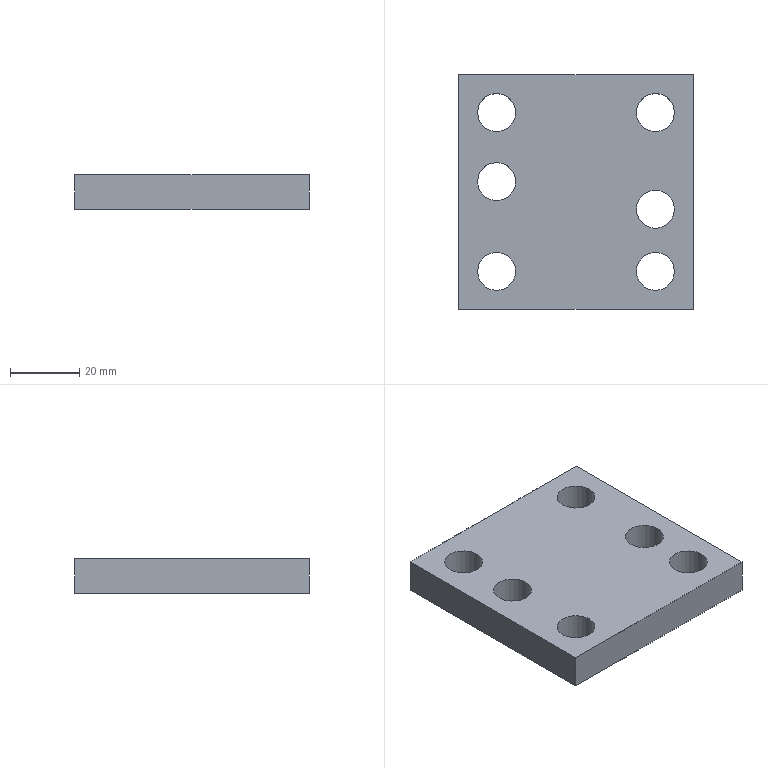Part | NX | features solid 2 | 1 solid | 12 faces | box 68 x 68 x 10 mm | volume 40538 mm3 | plane 6 | cylinder 6 | commonest cylinder face diameters 11 x6
STEP:
#1=CARTESIAN_POINT('',(1122.079,-107.904,88.));
#2=VERTEX_POINT('',#1);
#3=CARTESIAN_POINT('',(1122.079,-107.904,78.));
#4=VERTEX_POINT('',#3);
#5=CARTESIAN_POINT('',(1122.079,-107.904,78.));
#6=DIRECTION('',(0.,0.,1.));
#7=VECTOR('',#6,1000.);
#8=LINE('',#5,#7);
#9=EDGE_CURVE('',#2,#4,#8,.F.);
#10=ORIENTED_EDGE('',*,*,#9,.T.);
#11=CARTESIAN_POINT('',(1054.079,-107.904,78.));
#12=VERTEX_POINT('',#11);
#13=CARTESIAN_POINT('',(1088.079,-107.904,78.));
#14=DIRECTION('',(-1.,0.,0.));
#15=VECTOR('',#14,1000.);
#16=LINE('',#13,#15);
#17=EDGE_CURVE('',#12,#4,#16,.F.);
#18=ORIENTED_EDGE('',*,*,#17,.F.);
#19=CARTESIAN_POINT('',(1054.079,-107.904,88.));
#20=VERTEX_POINT('',#19);
#21=CARTESIAN_POINT('',(1054.079,-107.904,78.));
#22=DIRECTION('',(0.,0.,1.));
#23=VECTOR('',#22,1000.);
#24=LINE('',#21,#23);
#25=EDGE_CURVE('',#20,#12,#24,.F.);
#26=ORIENTED_EDGE('',*,*,#25,.F.);
#27=CARTESIAN_POINT('',(287.,-107.904,88.));
#28=DIRECTION('',(-1.,0.,0.));
#29=VECTOR('',#28,1000.);
#30=LINE('',#27,#29);
#31=EDGE_CURVE('',#20,#2,#30,.F.);
#32=ORIENTED_EDGE('',*,*,#31,.T.);
#33=EDGE_LOOP('',(#10,#18,#26,#32));
#34=FACE_BOUND('',#33,.T.);
#35=CARTESIAN_POINT('',(1088.079,-107.904,78.));
#36=DIRECTION('',(0.,-1.,0.));
#37=DIRECTION('',(-1.,0.,0.));
#38=AXIS2_PLACEMENT_3D('',#35,#36,#37);
#39=PLANE('',#38);
#40=ADVANCED_FACE('',(#34),#39,.F.);
#41=ORIENTED_EDGE('',*,*,#25,.T.);
#42=CARTESIAN_POINT('',(1054.079,-175.904,78.));
#43=VERTEX_POINT('',#42);
#44=CARTESIAN_POINT('',(1054.079,-141.904,78.));
#45=DIRECTION('',(0.,-1.,0.));
#46=VECTOR('',#45,1000.);
#47=LINE('',#44,#46);
#48=EDGE_CURVE('',#43,#12,#47,.F.);
#49=ORIENTED_EDGE('',*,*,#48,.F.);
#50=CARTESIAN_POINT('',(1054.079,-175.904,88.));
#51=VERTEX_POINT('',#50);
#52=CARTESIAN_POINT('',(1054.079,-175.904,78.));
#53=DIRECTION('',(0.,0.,1.));
#54=VECTOR('',#53,1000.);
#55=LINE('',#52,#54);
#56=EDGE_CURVE('',#51,#43,#55,.F.);
#57=ORIENTED_EDGE('',*,*,#56,.F.);
#58=CARTESIAN_POINT('',(1054.079,-0.000000688,88.));
#59=DIRECTION('',(0.,1.,0.));
#60=VECTOR('',#59,1000.);
#61=LINE('',#58,#60);
#62=EDGE_CURVE('',#51,#20,#61,.T.);
#63=ORIENTED_EDGE('',*,*,#62,.T.);
#64=EDGE_LOOP('',(#41,#49,#57,#63));
#65=FACE_BOUND('',#64,.T.);
#66=CARTESIAN_POINT('',(1054.079,-141.904,78.));
#67=DIRECTION('',(1.,0.,0.));
#68=DIRECTION('',(0.,-1.,0.));
#69=AXIS2_PLACEMENT_3D('',#66,#67,#68);
#70=PLANE('',#69);
#71=ADVANCED_FACE('',(#65),#70,.F.);
#72=ORIENTED_EDGE('',*,*,#56,.T.);
#73=CARTESIAN_POINT('',(1122.079,-175.904,78.));
#74=VERTEX_POINT('',#73);
#75=CARTESIAN_POINT('',(1088.079,-175.904,78.));
#76=DIRECTION('',(1.,0.,0.));
#77=VECTOR('',#76,1000.);
#78=LINE('',#75,#77);
#79=EDGE_CURVE('',#74,#43,#78,.F.);
#80=ORIENTED_EDGE('',*,*,#79,.F.);
#81=CARTESIAN_POINT('',(1122.079,-175.904,88.));
#82=VERTEX_POINT('',#81);
#83=CARTESIAN_POINT('',(1122.079,-175.904,78.));
#84=DIRECTION('',(0.,0.,1.));
#85=VECTOR('',#84,1000.);
#86=LINE('',#83,#85);
#87=EDGE_CURVE('',#82,#74,#86,.F.);
#88=ORIENTED_EDGE('',*,*,#87,.F.);
#89=CARTESIAN_POINT('',(287.,-175.904,88.));
#90=DIRECTION('',(-1.,0.,0.));
#91=VECTOR('',#90,1000.);
#92=LINE('',#89,#91);
#93=EDGE_CURVE('',#82,#51,#92,.T.);
#94=ORIENTED_EDGE('',*,*,#93,.T.);
#95=EDGE_LOOP('',(#72,#80,#88,#94));
#96=FACE_BOUND('',#95,.T.);
#97=CARTESIAN_POINT('',(1088.079,-175.904,78.));
#98=DIRECTION('',(0.,1.,0.));
#99=DIRECTION('',(1.,0.,0.));
#100=AXIS2_PLACEMENT_3D('',#97,#98,#99);
#101=PLANE('',#100);
#102=ADVANCED_FACE('',(#96),#101,.F.);
#103=CARTESIAN_POINT('',(1105.579,-146.904,78.));
#104=VERTEX_POINT('',#103);
#105=CARTESIAN_POINT('',(1111.079,-146.904,78.));
#106=DIRECTION('',(0.,0.,-1.));
#107=DIRECTION('',(-1.,0.,0.));
#108=AXIS2_PLACEMENT_3D('',#105,#106,#107);
#109=CIRCLE('',#108,5.5);
#110=EDGE_CURVE('',#104,#104,#109,.T.);
#111=ORIENTED_EDGE('',*,*,#110,.T.);
#112=EDGE_LOOP('',(#111));
#113=FACE_BOUND('',#112,.T.);
#114=CARTESIAN_POINT('',(1105.579,-146.904,88.));
#115=VERTEX_POINT('',#114);
#116=CARTESIAN_POINT('',(1111.079,-146.904,88.));
#117=DIRECTION('',(0.,0.,-1.));
#118=DIRECTION('',(-1.,0.,0.));
#119=AXIS2_PLACEMENT_3D('',#116,#117,#118);
#120=CIRCLE('',#119,5.5);
#121=EDGE_CURVE('',#115,#115,#120,.T.);
#122=ORIENTED_EDGE('',*,*,#121,.F.);
#123=EDGE_LOOP('',(#122));
#124=FACE_BOUND('',#123,.T.);
#125=CARTESIAN_POINT('',(1111.079,-146.904,78.));
#126=DIRECTION('',(0.,0.,-1.));
#127=DIRECTION('',(-1.,0.,0.));
#128=AXIS2_PLACEMENT_3D('',#125,#126,#127);
#129=CYLINDRICAL_SURFACE('',#128,5.5);
#130=ADVANCED_FACE('',(#113,#124),#129,.F.);
#131=CARTESIAN_POINT('',(1059.579,-138.904,78.));
#132=VERTEX_POINT('',#131);
#133=CARTESIAN_POINT('',(1065.079,-138.904,78.));
#134=DIRECTION('',(0.,0.,-1.));
#135=DIRECTION('',(-1.,0.,0.));
#136=AXIS2_PLACEMENT_3D('',#133,#134,#135);
#137=CIRCLE('',#136,5.5);
#138=EDGE_CURVE('',#132,#132,#137,.F.);
#139=ORIENTED_EDGE('',*,*,#138,.F.);
#140=EDGE_LOOP('',(#139));
#141=FACE_BOUND('',#140,.T.);
#142=CARTESIAN_POINT('',(1059.579,-138.904,88.));
#143=VERTEX_POINT('',#142);
#144=CARTESIAN_POINT('',(1065.079,-138.904,88.));
#145=DIRECTION('',(0.,0.,-1.));
#146=DIRECTION('',(-1.,0.,0.));
#147=AXIS2_PLACEMENT_3D('',#144,#145,#146);
#148=CIRCLE('',#147,5.5);
#149=EDGE_CURVE('',#143,#143,#148,.F.);
#150=ORIENTED_EDGE('',*,*,#149,.T.);
#151=EDGE_LOOP('',(#150));
#152=FACE_BOUND('',#151,.T.);
#153=CARTESIAN_POINT('',(1065.079,-138.904,78.));
#154=DIRECTION('',(0.,0.,-1.));
#155=DIRECTION('',(-1.,0.,0.));
#156=AXIS2_PLACEMENT_3D('',#153,#154,#155);
#157=CYLINDRICAL_SURFACE('',#156,5.5);
#158=ADVANCED_FACE('',(#141,#152),#157,.F.);
#159=CARTESIAN_POINT('',(1105.579,-118.904,78.));
#160=VERTEX_POINT('',#159);
#161=CARTESIAN_POINT('',(1111.079,-118.904,78.));
#162=DIRECTION('',(0.,0.,-1.));
#163=DIRECTION('',(-1.,0.,0.));
#164=AXIS2_PLACEMENT_3D('',#161,#162,#163);
#165=CIRCLE('',#164,5.5);
#166=EDGE_CURVE('',#160,#160,#165,.T.);
#167=ORIENTED_EDGE('',*,*,#166,.T.);
#168=EDGE_LOOP('',(#167));
#169=FACE_BOUND('',#168,.T.);
#170=CARTESIAN_POINT('',(1105.579,-118.904,88.));
#171=VERTEX_POINT('',#170);
#172=CARTESIAN_POINT('',(1111.079,-118.904,88.));
#173=DIRECTION('',(0.,0.,-1.));
#174=DIRECTION('',(-1.,0.,0.));
#175=AXIS2_PLACEMENT_3D('',#172,#173,#174);
#176=CIRCLE('',#175,5.5);
#177=EDGE_CURVE('',#171,#171,#176,.T.);
#178=ORIENTED_EDGE('',*,*,#177,.F.);
#179=EDGE_LOOP('',(#178));
#180=FACE_BOUND('',#179,.T.);
#181=CARTESIAN_POINT('',(1111.079,-118.904,78.));
#182=DIRECTION('',(0.,0.,-1.));
#183=DIRECTION('',(-1.,0.,0.));
#184=AXIS2_PLACEMENT_3D('',#181,#182,#183);
#185=CYLINDRICAL_SURFACE('',#184,5.5);
#186=ADVANCED_FACE('',(#169,#180),#185,.F.);
#187=CARTESIAN_POINT('',(1105.579,-164.904,78.));
#188=VERTEX_POINT('',#187);
#189=CARTESIAN_POINT('',(1111.079,-164.904,78.));
#190=DIRECTION('',(0.,0.,-1.));
#191=DIRECTION('',(-1.,0.,0.));
#192=AXIS2_PLACEMENT_3D('',#189,#190,#191);
#193=CIRCLE('',#192,5.5);
#194=EDGE_CURVE('',#188,#188,#193,.T.);
#195=ORIENTED_EDGE('',*,*,#194,.T.);
#196=EDGE_LOOP('',(#195));
#197=FACE_BOUND('',#196,.T.);
#198=CARTESIAN_POINT('',(1105.579,-164.904,88.));
#199=VERTEX_POINT('',#198);
#200=CARTESIAN_POINT('',(1111.079,-164.904,88.));
#201=DIRECTION('',(0.,0.,-1.));
#202=DIRECTION('',(-1.,0.,0.));
#203=AXIS2_PLACEMENT_3D('',#200,#201,#202);
#204=CIRCLE('',#203,5.5);
#205=EDGE_CURVE('',#199,#199,#204,.T.);
#206=ORIENTED_EDGE('',*,*,#205,.F.);
#207=EDGE_LOOP('',(#206));
#208=FACE_BOUND('',#207,.T.);
#209=CARTESIAN_POINT('',(1111.079,-164.904,78.));
#210=DIRECTION('',(0.,0.,-1.));
#211=DIRECTION('',(-1.,0.,0.));
#212=AXIS2_PLACEMENT_3D('',#209,#210,#211);
#213=CYLINDRICAL_SURFACE('',#212,5.5);
#214=ADVANCED_FACE('',(#197,#208),#213,.F.);
#215=CARTESIAN_POINT('',(1059.579,-164.904,78.));
#216=VERTEX_POINT('',#215);
#217=CARTESIAN_POINT('',(1065.079,-164.904,78.));
#218=DIRECTION('',(0.,0.,-1.));
#219=DIRECTION('',(-1.,0.,0.));
#220=AXIS2_PLACEMENT_3D('',#217,#218,#219);
#221=CIRCLE('',#220,5.5);
#222=EDGE_CURVE('',#216,#216,#221,.T.);
#223=ORIENTED_EDGE('',*,*,#222,.T.);
#224=EDGE_LOOP('',(#223));
#225=FACE_BOUND('',#224,.T.);
#226=CARTESIAN_POINT('',(1059.579,-164.904,88.));
#227=VERTEX_POINT('',#226);
#228=CARTESIAN_POINT('',(1065.079,-164.904,88.));
#229=DIRECTION('',(0.,0.,-1.));
#230=DIRECTION('',(-1.,0.,0.));
#231=AXIS2_PLACEMENT_3D('',#228,#229,#230);
#232=CIRCLE('',#231,5.5);
#233=EDGE_CURVE('',#227,#227,#232,.T.);
#234=ORIENTED_EDGE('',*,*,#233,.F.);
#235=EDGE_LOOP('',(#234));
#236=FACE_BOUND('',#235,.T.);
#237=CARTESIAN_POINT('',(1065.079,-164.904,78.));
#238=DIRECTION('',(0.,0.,-1.));
#239=DIRECTION('',(-1.,0.,0.));
#240=AXIS2_PLACEMENT_3D('',#237,#238,#239);
#241=CYLINDRICAL_SURFACE('',#240,5.5);
#242=ADVANCED_FACE('',(#225,#236),#241,.F.);
#243=CARTESIAN_POINT('',(1059.579,-118.904,78.));
#244=VERTEX_POINT('',#243);
#245=CARTESIAN_POINT('',(1065.079,-118.904,78.));
#246=DIRECTION('',(0.,0.,-1.));
#247=DIRECTION('',(-1.,0.,0.));
#248=AXIS2_PLACEMENT_3D('',#245,#246,#247);
#249=CIRCLE('',#248,5.5);
#250=EDGE_CURVE('',#244,#244,#249,.F.);
#251=ORIENTED_EDGE('',*,*,#250,.F.);
#252=EDGE_LOOP('',(#251));
#253=FACE_BOUND('',#252,.T.);
#254=CARTESIAN_POINT('',(1059.579,-118.904,88.));
#255=VERTEX_POINT('',#254);
#256=CARTESIAN_POINT('',(1065.079,-118.904,88.));
#257=DIRECTION('',(0.,0.,-1.));
#258=DIRECTION('',(-1.,0.,0.));
#259=AXIS2_PLACEMENT_3D('',#256,#257,#258);
#260=CIRCLE('',#259,5.5);
#261=EDGE_CURVE('',#255,#255,#260,.F.);
#262=ORIENTED_EDGE('',*,*,#261,.T.);
#263=EDGE_LOOP('',(#262));
#264=FACE_BOUND('',#263,.T.);
#265=CARTESIAN_POINT('',(1065.079,-118.904,78.));
#266=DIRECTION('',(0.,0.,-1.));
#267=DIRECTION('',(-1.,0.,0.));
#268=AXIS2_PLACEMENT_3D('',#265,#266,#267);
#269=CYLINDRICAL_SURFACE('',#268,5.5);
#270=ADVANCED_FACE('',(#253,#264),#269,.F.);
#271=CARTESIAN_POINT('',(1122.079,-0.000000688,88.));
#272=DIRECTION('',(0.,1.,0.));
#273=VECTOR('',#272,1000.);
#274=LINE('',#271,#273);
#275=EDGE_CURVE('',#2,#82,#274,.F.);
#276=ORIENTED_EDGE('',*,*,#275,.T.);
#277=ORIENTED_EDGE('',*,*,#87,.T.);
#278=CARTESIAN_POINT('',(1122.079,-141.904,78.));
#279=DIRECTION('',(0.,1.,0.));
#280=VECTOR('',#279,1000.);
#281=LINE('',#278,#280);
#282=EDGE_CURVE('',#4,#74,#281,.F.);
#283=ORIENTED_EDGE('',*,*,#282,.F.);
#284=ORIENTED_EDGE('',*,*,#9,.F.);
#285=EDGE_LOOP('',(#276,#277,#283,#284));
#286=FACE_BOUND('',#285,.T.);
#287=CARTESIAN_POINT('',(1122.079,-141.904,78.));
#288=DIRECTION('',(-1.,0.,0.));
#289=DIRECTION('',(0.,1.,0.));
#290=AXIS2_PLACEMENT_3D('',#287,#288,#289);
#291=PLANE('',#290);
#292=ADVANCED_FACE('',(#286),#291,.F.);
#293=ORIENTED_EDGE('',*,*,#110,.F.);
#294=EDGE_LOOP('',(#293));
#295=FACE_BOUND('',#294,.T.);
#296=ORIENTED_EDGE('',*,*,#138,.T.);
#297=EDGE_LOOP('',(#296));
#298=FACE_BOUND('',#297,.T.);
#299=ORIENTED_EDGE('',*,*,#166,.F.);
#300=EDGE_LOOP('',(#299));
#301=FACE_BOUND('',#300,.T.);
#302=ORIENTED_EDGE('',*,*,#194,.F.);
#303=EDGE_LOOP('',(#302));
#304=FACE_BOUND('',#303,.T.);
#305=ORIENTED_EDGE('',*,*,#222,.F.);
#306=EDGE_LOOP('',(#305));
#307=FACE_BOUND('',#306,.T.);
#308=ORIENTED_EDGE('',*,*,#250,.T.);
#309=EDGE_LOOP('',(#308));
#310=FACE_BOUND('',#309,.T.);
#311=ORIENTED_EDGE('',*,*,#79,.T.);
#312=ORIENTED_EDGE('',*,*,#48,.T.);
#313=ORIENTED_EDGE('',*,*,#17,.T.);
#314=ORIENTED_EDGE('',*,*,#282,.T.);
#315=EDGE_LOOP('',(#311,#312,#313,#314));
#316=FACE_BOUND('',#315,.T.);
#317=CARTESIAN_POINT('',(287.,-0.000000688,78.));
#318=DIRECTION('',(0.,0.,-1.));
#319=DIRECTION('',(-1.,0.,0.));
#320=AXIS2_PLACEMENT_3D('',#317,#318,#319);
#321=PLANE('',#320);
#322=ADVANCED_FACE('',(#295,#298,#301,#304,#307,#310,#316),#321,.T.);
#323=ORIENTED_EDGE('',*,*,#121,.T.);
#324=EDGE_LOOP('',(#323));
#325=FACE_BOUND('',#324,.T.);
#326=ORIENTED_EDGE('',*,*,#149,.F.);
#327=EDGE_LOOP('',(#326));
#328=FACE_BOUND('',#327,.T.);
#329=ORIENTED_EDGE('',*,*,#177,.T.);
#330=EDGE_LOOP('',(#329));
#331=FACE_BOUND('',#330,.T.);
#332=ORIENTED_EDGE('',*,*,#205,.T.);
#333=EDGE_LOOP('',(#332));
#334=FACE_BOUND('',#333,.T.);
#335=ORIENTED_EDGE('',*,*,#233,.T.);
#336=EDGE_LOOP('',(#335));
#337=FACE_BOUND('',#336,.T.);
#338=ORIENTED_EDGE('',*,*,#261,.F.);
#339=EDGE_LOOP('',(#338));
#340=FACE_BOUND('',#339,.T.);
#341=ORIENTED_EDGE('',*,*,#93,.F.);
#342=ORIENTED_EDGE('',*,*,#275,.F.);
#343=ORIENTED_EDGE('',*,*,#31,.F.);
#344=ORIENTED_EDGE('',*,*,#62,.F.);
#345=EDGE_LOOP('',(#341,#342,#343,#344));
#346=FACE_BOUND('',#345,.T.);
#347=CARTESIAN_POINT('',(287.,-0.000000688,88.));
#348=DIRECTION('',(0.,0.,-1.));
#349=DIRECTION('',(-1.,0.,0.));
#350=AXIS2_PLACEMENT_3D('',#347,#348,#349);
#351=PLANE('',#350);
#352=ADVANCED_FACE('',(#325,#328,#331,#334,#337,#340,#346),#351,.F.);
#353=CLOSED_SHELL('',(#40,#71,#102,#130,#158,#186,#214,#242,#270,#292,#322,#352));
#354=MANIFOLD_SOLID_BREP('',#353);
#355=(LENGTH_UNIT()NAMED_UNIT(*)SI_UNIT(.MILLI.,.METRE.));
#356=UNCERTAINTY_MEASURE_WITH_UNIT(LENGTH_MEASURE(0.00001),#355,'','');
#357=(NAMED_UNIT(*)PLANE_ANGLE_UNIT()SI_UNIT($,.RADIAN.));
#358=(NAMED_UNIT(*)SI_UNIT($,.STERADIAN.)SOLID_ANGLE_UNIT());
#359=(GEOMETRIC_REPRESENTATION_CONTEXT(3)GLOBAL_UNCERTAINTY_ASSIGNED_CONTEXT((#356))GLOBAL_UNIT_ASSIGNED_CONTEXT((#355,#357,#358))REPRESENTATION_CONTEXT('',''));
#360=ADVANCED_BREP_SHAPE_REPRESENTATION('',(#354),#359);